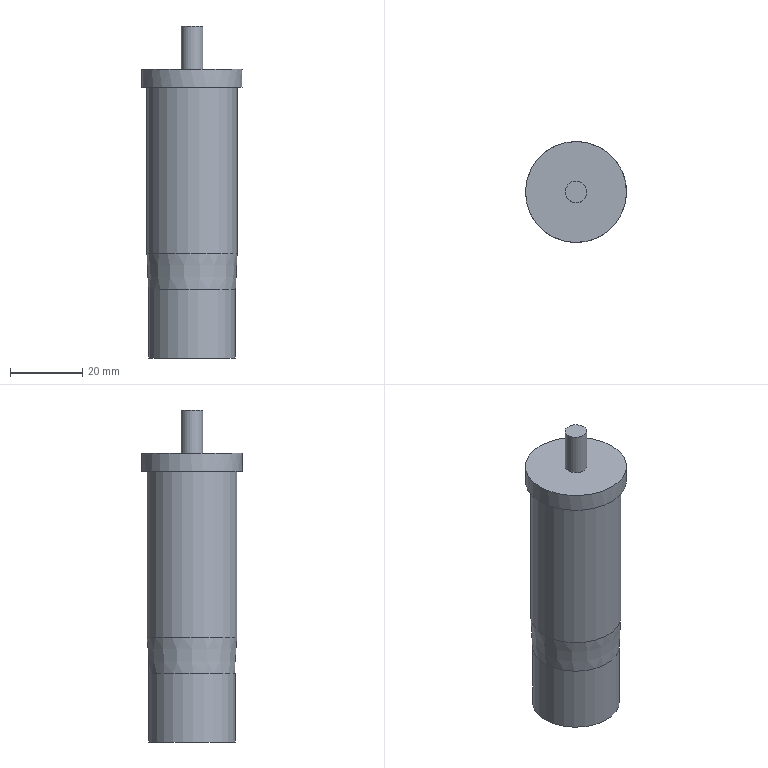Part | NX | features solid 2 | 1 solid | 9 faces | box 28 x 28 x 92 mm | volume 39400 mm3 | plane 4 | cylinder 4 | cone 1 | commonest cylinder face diameters 6 x1 24.1 x1 25 x1 28 x1
STEP:
#1=CARTESIAN_POINT('',(265.756,1.566,30.));
#2=VERTEX_POINT('',#1);
#3=CARTESIAN_POINT('',(274.986,-6.179,30.));
#4=DIRECTION('',(0.,0.,-1.));
#5=DIRECTION('',(-0.766,0.6428,0.));
#6=AXIS2_PLACEMENT_3D('',#3,#4,#5);
#7=CIRCLE('',#6,12.05);
#8=EDGE_CURVE('',#2,#2,#7,.T.);
#9=ORIENTED_EDGE('',*,*,#8,.T.);
#10=EDGE_LOOP('',(#9));
#11=FACE_BOUND('',#10,.T.);
#12=CARTESIAN_POINT('',(274.986,-6.179,30.));
#13=DIRECTION('',(0.,0.,-1.));
#14=DIRECTION('',(0.766,-0.6428,0.));
#15=AXIS2_PLACEMENT_3D('',#12,#13,#14);
#16=PLANE('',#15);
#17=ADVANCED_FACE('',(#11),#16,.T.);
#18=CARTESIAN_POINT('',(265.756,1.566,49.));
#19=VERTEX_POINT('',#18);
#20=CARTESIAN_POINT('',(274.986,-6.179,49.));
#21=DIRECTION('',(0.,0.,-1.));
#22=DIRECTION('',(-0.766,0.6428,0.));
#23=AXIS2_PLACEMENT_3D('',#20,#21,#22);
#24=CIRCLE('',#23,12.05);
#25=EDGE_CURVE('',#19,#19,#24,.T.);
#26=ORIENTED_EDGE('',*,*,#25,.T.);
#27=EDGE_LOOP('',(#26));
#28=FACE_BOUND('',#27,.T.);
#29=ORIENTED_EDGE('',*,*,#8,.F.);
#30=EDGE_LOOP('',(#29));
#31=FACE_BOUND('',#30,.T.);
#32=CARTESIAN_POINT('',(274.986,-6.179,30.));
#33=DIRECTION('',(0.,0.,1.));
#34=DIRECTION('',(-0.766,0.6428,0.));
#35=AXIS2_PLACEMENT_3D('',#32,#33,#34);
#36=CYLINDRICAL_SURFACE('',#35,12.05);
#37=ADVANCED_FACE('',(#28,#31),#36,.T.);
#38=ORIENTED_EDGE('',*,*,#25,.F.);
#39=EDGE_LOOP('',(#38));
#40=FACE_BOUND('',#39,.T.);
#41=CARTESIAN_POINT('',(265.411,1.856,59.));
#42=VERTEX_POINT('',#41);
#43=CARTESIAN_POINT('',(274.986,-6.179,59.));
#44=DIRECTION('',(0.,0.,-1.));
#45=DIRECTION('',(-0.766,0.6428,0.));
#46=AXIS2_PLACEMENT_3D('',#43,#44,#45);
#47=CIRCLE('',#46,12.5);
#48=EDGE_CURVE('',#42,#42,#47,.T.);
#49=ORIENTED_EDGE('',*,*,#48,.T.);
#50=EDGE_LOOP('',(#49));
#51=FACE_BOUND('',#50,.T.);
#52=CARTESIAN_POINT('',(274.986,-6.179,49.));
#53=DIRECTION('',(0.,0.,1.));
#54=DIRECTION('',(-0.766,0.6428,0.));
#55=AXIS2_PLACEMENT_3D('',#52,#53,#54);
#56=CONICAL_SURFACE('',#55,12.05,0.04497);
#57=ADVANCED_FACE('',(#40,#51),#56,.T.);
#58=CARTESIAN_POINT('',(284.562,-14.214,105.));
#59=VERTEX_POINT('',#58);
#60=CARTESIAN_POINT('',(274.986,-6.179,105.));
#61=DIRECTION('',(0.,0.,1.));
#62=DIRECTION('',(0.766,-0.6428,0.));
#63=AXIS2_PLACEMENT_3D('',#60,#61,#62);
#64=CIRCLE('',#63,12.5);
#65=EDGE_CURVE('',#59,#59,#64,.F.);
#66=ORIENTED_EDGE('',*,*,#65,.T.);
#67=EDGE_LOOP('',(#66));
#68=FACE_BOUND('',#67,.T.);
#69=ORIENTED_EDGE('',*,*,#48,.F.);
#70=EDGE_LOOP('',(#69));
#71=FACE_BOUND('',#70,.T.);
#72=CARTESIAN_POINT('',(274.986,-6.179,59.));
#73=DIRECTION('',(0.,0.,1.));
#74=DIRECTION('',(-0.766,0.6428,0.));
#75=AXIS2_PLACEMENT_3D('',#72,#73,#74);
#76=CYLINDRICAL_SURFACE('',#75,12.5);
#77=ADVANCED_FACE('',(#68,#71),#76,.T.);
#78=CARTESIAN_POINT('',(272.688,-4.251,110.));
#79=VERTEX_POINT('',#78);
#80=CARTESIAN_POINT('',(274.986,-6.179,110.));
#81=DIRECTION('',(0.,0.,-1.));
#82=DIRECTION('',(-0.766,0.6428,0.));
#83=AXIS2_PLACEMENT_3D('',#80,#81,#82);
#84=CIRCLE('',#83,3.);
#85=EDGE_CURVE('',#79,#79,#84,.T.);
#86=ORIENTED_EDGE('',*,*,#85,.T.);
#87=EDGE_LOOP('',(#86));
#88=FACE_BOUND('',#87,.T.);
#89=CARTESIAN_POINT('',(285.711,-15.178,110.));
#90=VERTEX_POINT('',#89);
#91=CARTESIAN_POINT('',(274.986,-6.179,110.));
#92=DIRECTION('',(0.,0.,1.));
#93=DIRECTION('',(0.766,-0.6428,0.));
#94=AXIS2_PLACEMENT_3D('',#91,#92,#93);
#95=CIRCLE('',#94,14.);
#96=EDGE_CURVE('',#90,#90,#95,.T.);
#97=ORIENTED_EDGE('',*,*,#96,.T.);
#98=EDGE_LOOP('',(#97));
#99=FACE_BOUND('',#98,.T.);
#100=CARTESIAN_POINT('',(274.986,-6.179,110.));
#101=DIRECTION('',(0.,0.,1.));
#102=DIRECTION('',(-0.766,0.6428,0.));
#103=AXIS2_PLACEMENT_3D('',#100,#101,#102);
#104=PLANE('',#103);
#105=ADVANCED_FACE('',(#88,#99),#104,.T.);
#106=ORIENTED_EDGE('',*,*,#65,.F.);
#107=EDGE_LOOP('',(#106));
#108=FACE_BOUND('',#107,.T.);
#109=CARTESIAN_POINT('',(264.262,2.82,105.));
#110=VERTEX_POINT('',#109);
#111=CARTESIAN_POINT('',(274.986,-6.179,105.));
#112=DIRECTION('',(0.,0.,-1.));
#113=DIRECTION('',(-0.766,0.6428,0.));
#114=AXIS2_PLACEMENT_3D('',#111,#112,#113);
#115=CIRCLE('',#114,14.);
#116=EDGE_CURVE('',#110,#110,#115,.T.);
#117=ORIENTED_EDGE('',*,*,#116,.T.);
#118=EDGE_LOOP('',(#117));
#119=FACE_BOUND('',#118,.T.);
#120=CARTESIAN_POINT('',(274.986,-6.179,105.));
#121=DIRECTION('',(0.,0.,-1.));
#122=DIRECTION('',(0.766,-0.6428,0.));
#123=AXIS2_PLACEMENT_3D('',#120,#121,#122);
#124=PLANE('',#123);
#125=ADVANCED_FACE('',(#108,#119),#124,.T.);
#126=ORIENTED_EDGE('',*,*,#96,.F.);
#127=EDGE_LOOP('',(#126));
#128=FACE_BOUND('',#127,.T.);
#129=ORIENTED_EDGE('',*,*,#116,.F.);
#130=EDGE_LOOP('',(#129));
#131=FACE_BOUND('',#130,.T.);
#132=CARTESIAN_POINT('',(274.986,-6.179,105.));
#133=DIRECTION('',(0.,0.,1.));
#134=DIRECTION('',(-0.766,0.6428,0.));
#135=AXIS2_PLACEMENT_3D('',#132,#133,#134);
#136=CYLINDRICAL_SURFACE('',#135,14.);
#137=ADVANCED_FACE('',(#128,#131),#136,.T.);
#138=CARTESIAN_POINT('',(277.285,-8.107,122.));
#139=VERTEX_POINT('',#138);
#140=CARTESIAN_POINT('',(274.986,-6.179,122.));
#141=DIRECTION('',(0.,0.,1.));
#142=DIRECTION('',(0.766,-0.6428,0.));
#143=AXIS2_PLACEMENT_3D('',#140,#141,#142);
#144=CIRCLE('',#143,3.);
#145=EDGE_CURVE('',#139,#139,#144,.T.);
#146=ORIENTED_EDGE('',*,*,#145,.T.);
#147=EDGE_LOOP('',(#146));
#148=FACE_BOUND('',#147,.T.);
#149=CARTESIAN_POINT('',(274.986,-6.179,122.));
#150=DIRECTION('',(0.,0.,1.));
#151=DIRECTION('',(-0.766,0.6428,0.));
#152=AXIS2_PLACEMENT_3D('',#149,#150,#151);
#153=PLANE('',#152);
#154=ADVANCED_FACE('',(#148),#153,.T.);
#155=ORIENTED_EDGE('',*,*,#145,.F.);
#156=EDGE_LOOP('',(#155));
#157=FACE_BOUND('',#156,.T.);
#158=ORIENTED_EDGE('',*,*,#85,.F.);
#159=EDGE_LOOP('',(#158));
#160=FACE_BOUND('',#159,.T.);
#161=CARTESIAN_POINT('',(274.986,-6.179,110.));
#162=DIRECTION('',(0.,0.,1.));
#163=DIRECTION('',(-0.766,0.6428,0.));
#164=AXIS2_PLACEMENT_3D('',#161,#162,#163);
#165=CYLINDRICAL_SURFACE('',#164,3.);
#166=ADVANCED_FACE('',(#157,#160),#165,.T.);
#167=CLOSED_SHELL('',(#17,#37,#57,#77,#105,#125,#137,#154,#166));
#168=MANIFOLD_SOLID_BREP('',#167);
#169=(LENGTH_UNIT()NAMED_UNIT(*)SI_UNIT(.MILLI.,.METRE.));
#170=UNCERTAINTY_MEASURE_WITH_UNIT(LENGTH_MEASURE(0.00001),#169,'','');
#171=(NAMED_UNIT(*)PLANE_ANGLE_UNIT()SI_UNIT($,.RADIAN.));
#172=(NAMED_UNIT(*)SI_UNIT($,.STERADIAN.)SOLID_ANGLE_UNIT());
#173=(GEOMETRIC_REPRESENTATION_CONTEXT(3)GLOBAL_UNCERTAINTY_ASSIGNED_CONTEXT((#170))GLOBAL_UNIT_ASSIGNED_CONTEXT((#169,#171,#172))REPRESENTATION_CONTEXT('',''));
#174=ADVANCED_BREP_SHAPE_REPRESENTATION('',(#168),#173);